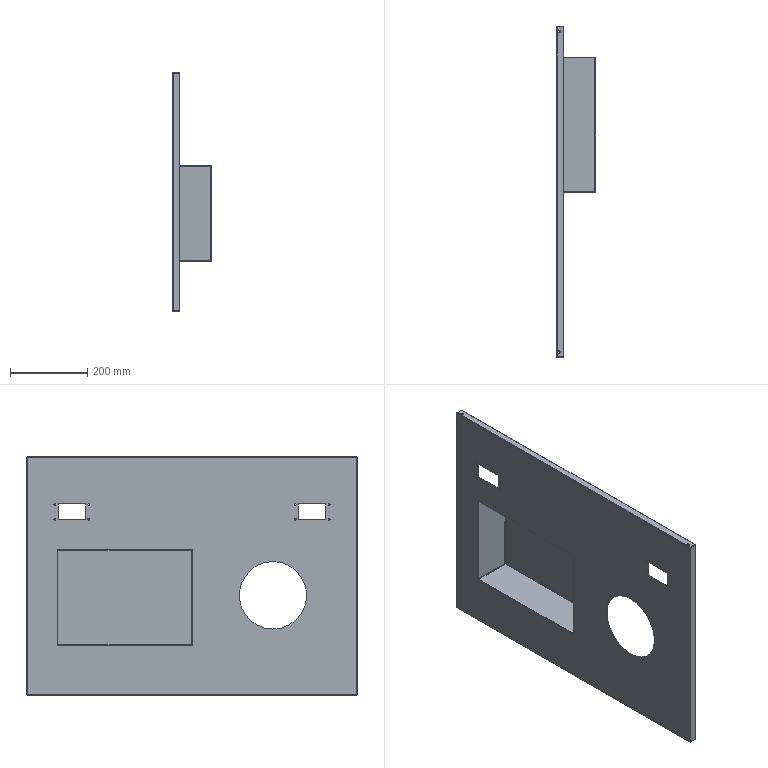Part | STEP file | 2 solids | 114 faces | box 101.5 x 858 x 618 mm | volume 647667 mm3 | plane 56 | cylinder 42 | spline 16 | commonest cylinder face diameters 5 x16 1.473 x8 7 x8 2.946 x4 4.473 x4 175 x2